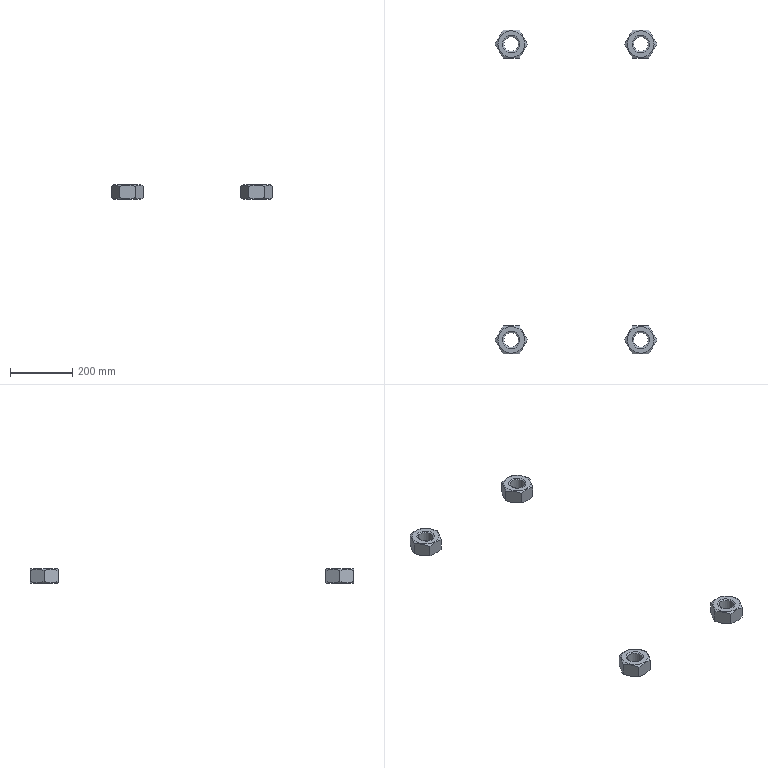Part | NX | features 4.SLDPRT 2, Delete Body 1, LINKED_BODY 1, SCALE 1 | 4 solids | 52 faces | box 520.173 x 1041 x 47.25 mm | volume 973230 mm3 | plane 32 | cone 16 | cylinder 4 | commonest cylinder face diameters 47.115 x4